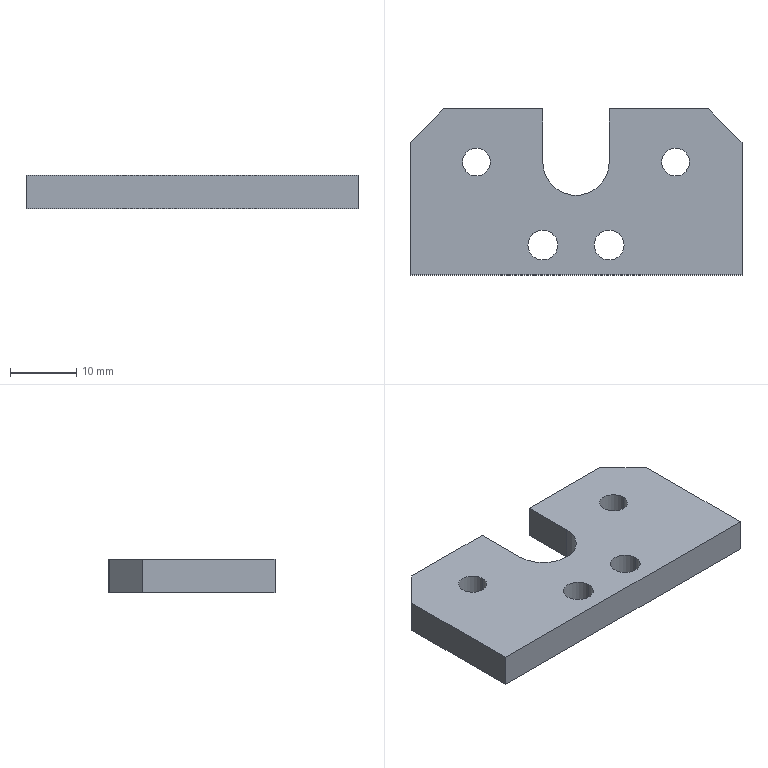Part | STEP file | BU-B05b | 1 solid | 20 faces | box 50 x 25 x 5 mm | volume 5231 mm3 | plane 11 | cylinder 9 | commonest cylinder face diameters 4.2 x4 4.5 x4 10 x1